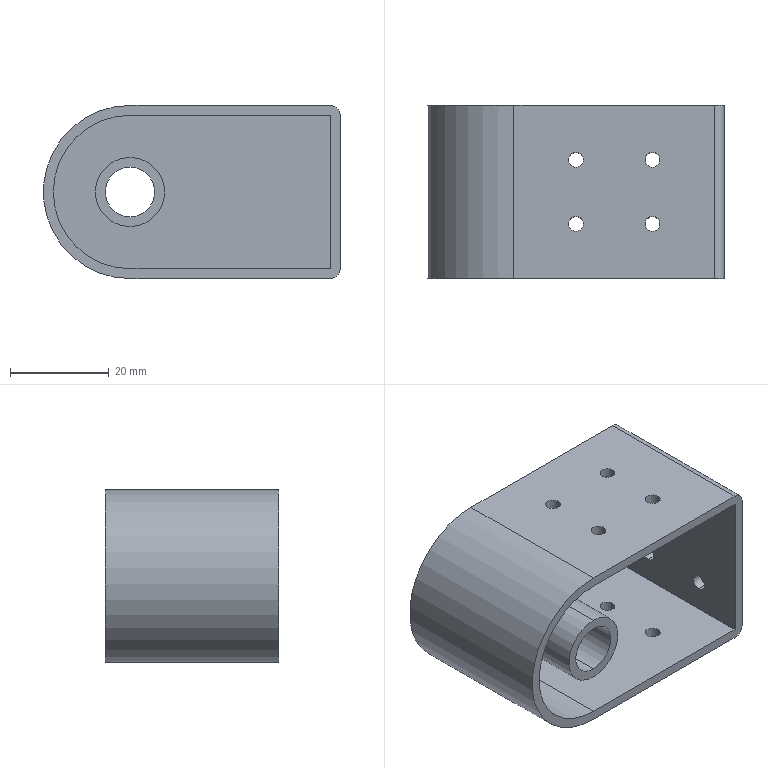Part | SolidWorks | features ICE 5, Extrusion 1, Fillet 1, Shell 1 | 1 solid | 42 faces | box 60 x 35 x 35 mm | volume 17116 mm3 | cylinder 32 | plane 10 | commonest cylinder face diameters 3 x24 4 x2 10 x2 14 x2 31 x1 35 x1
STEP:
#1=CARTESIAN_POINT('',(30.,24.748,-7.494));
#2=VERTEX_POINT('',#1);
#3=CARTESIAN_POINT('',(30.,24.748,-10.494));
#4=VERTEX_POINT('',#3);
#5=CARTESIAN_POINT('',(30.,24.748,-8.994));
#6=DIRECTION('',(1.,0.,0.));
#7=DIRECTION('',(0.,0.,1.));
#8=AXIS2_PLACEMENT_3D('',#5,#6,#7);
#9=CIRCLE('',#8,1.5);
#10=EDGE_CURVE('',#2,#4,#9,.T.);
#11=ORIENTED_EDGE('',*,*,#10,.T.);
#12=CARTESIAN_POINT('',(28.,24.748,-10.494));
#13=VERTEX_POINT('',#12);
#14=CARTESIAN_POINT('',(30.,24.748,-10.494));
#15=DIRECTION('',(-1.,0.,0.));
#16=VECTOR('',#15,1000.);
#17=LINE('',#14,#16);
#18=EDGE_CURVE('',#4,#13,#17,.T.);
#19=ORIENTED_EDGE('',*,*,#18,.T.);
#20=CARTESIAN_POINT('',(28.,24.748,-7.494));
#21=VERTEX_POINT('',#20);
#22=CARTESIAN_POINT('',(28.,24.748,-8.994));
#23=DIRECTION('',(1.,0.,0.));
#24=DIRECTION('',(0.,0.,1.));
#25=AXIS2_PLACEMENT_3D('',#22,#23,#24);
#26=CIRCLE('',#25,1.5);
#27=EDGE_CURVE('',#21,#13,#26,.T.);
#28=ORIENTED_EDGE('',*,*,#27,.F.);
#29=CARTESIAN_POINT('',(30.,24.748,-7.494));
#30=DIRECTION('',(-1.,0.,0.));
#31=VECTOR('',#30,1000.);
#32=LINE('',#29,#31);
#33=EDGE_CURVE('',#2,#21,#32,.T.);
#34=ORIENTED_EDGE('',*,*,#33,.F.);
#35=EDGE_LOOP('',(#11,#19,#28,#34));
#36=FACE_OUTER_BOUND('',#35,.T.);
#37=CARTESIAN_POINT('',(30.,24.748,-8.994));
#38=DIRECTION('',(-1.,0.,0.));
#39=DIRECTION('',(0.,0.,1.));
#40=AXIS2_PLACEMENT_3D('',#37,#38,#39);
#41=CYLINDRICAL_SURFACE('',#40,1.5);
#42=ADVANCED_FACE('',(#36),#41,.F.);
#43=CARTESIAN_POINT('',(30.,10.252,10.494));
#44=VERTEX_POINT('',#43);
#45=CARTESIAN_POINT('',(30.,10.252,7.494));
#46=VERTEX_POINT('',#45);
#47=CARTESIAN_POINT('',(30.,10.252,8.994));
#48=DIRECTION('',(1.,0.,0.));
#49=DIRECTION('',(0.,0.,1.));
#50=AXIS2_PLACEMENT_3D('',#47,#48,#49);
#51=CIRCLE('',#50,1.5);
#52=EDGE_CURVE('',#44,#46,#51,.T.);
#53=ORIENTED_EDGE('',*,*,#52,.T.);
#54=CARTESIAN_POINT('',(28.,10.252,7.494));
#55=VERTEX_POINT('',#54);
#56=CARTESIAN_POINT('',(30.,10.252,7.494));
#57=DIRECTION('',(-1.,0.,0.));
#58=VECTOR('',#57,1000.);
#59=LINE('',#56,#58);
#60=EDGE_CURVE('',#46,#55,#59,.T.);
#61=ORIENTED_EDGE('',*,*,#60,.T.);
#62=CARTESIAN_POINT('',(28.,10.252,10.494));
#63=VERTEX_POINT('',#62);
#64=CARTESIAN_POINT('',(28.,10.252,8.994));
#65=DIRECTION('',(1.,0.,0.));
#66=DIRECTION('',(0.,0.,1.));
#67=AXIS2_PLACEMENT_3D('',#64,#65,#66);
#68=CIRCLE('',#67,1.5);
#69=EDGE_CURVE('',#63,#55,#68,.T.);
#70=ORIENTED_EDGE('',*,*,#69,.F.);
#71=CARTESIAN_POINT('',(30.,10.252,10.494));
#72=DIRECTION('',(-1.,0.,0.));
#73=VECTOR('',#72,1000.);
#74=LINE('',#71,#73);
#75=EDGE_CURVE('',#44,#63,#74,.T.);
#76=ORIENTED_EDGE('',*,*,#75,.F.);
#77=EDGE_LOOP('',(#53,#61,#70,#76));
#78=FACE_OUTER_BOUND('',#77,.T.);
#79=CARTESIAN_POINT('',(30.,10.252,8.994));
#80=DIRECTION('',(-1.,0.,0.));
#81=DIRECTION('',(0.,0.,1.));
#82=AXIS2_PLACEMENT_3D('',#79,#80,#81);
#83=CYLINDRICAL_SURFACE('',#82,1.5);
#84=ADVANCED_FACE('',(#78),#83,.F.);
#85=CARTESIAN_POINT('',(30.,10.252,-7.494));
#86=VERTEX_POINT('',#85);
#87=CARTESIAN_POINT('',(30.,10.252,-10.494));
#88=VERTEX_POINT('',#87);
#89=CARTESIAN_POINT('',(30.,10.252,-8.994));
#90=DIRECTION('',(1.,0.,0.));
#91=DIRECTION('',(0.,0.,1.));
#92=AXIS2_PLACEMENT_3D('',#89,#90,#91);
#93=CIRCLE('',#92,1.5);
#94=EDGE_CURVE('',#86,#88,#93,.T.);
#95=ORIENTED_EDGE('',*,*,#94,.T.);
#96=CARTESIAN_POINT('',(28.,10.252,-10.494));
#97=VERTEX_POINT('',#96);
#98=CARTESIAN_POINT('',(30.,10.252,-10.494));
#99=DIRECTION('',(-1.,0.,0.));
#100=VECTOR('',#99,1000.);
#101=LINE('',#98,#100);
#102=EDGE_CURVE('',#88,#97,#101,.T.);
#103=ORIENTED_EDGE('',*,*,#102,.T.);
#104=CARTESIAN_POINT('',(28.,10.252,-7.494));
#105=VERTEX_POINT('',#104);
#106=CARTESIAN_POINT('',(28.,10.252,-8.994));
#107=DIRECTION('',(1.,0.,0.));
#108=DIRECTION('',(0.,0.,1.));
#109=AXIS2_PLACEMENT_3D('',#106,#107,#108);
#110=CIRCLE('',#109,1.5);
#111=EDGE_CURVE('',#105,#97,#110,.T.);
#112=ORIENTED_EDGE('',*,*,#111,.F.);
#113=CARTESIAN_POINT('',(30.,10.252,-7.494));
#114=DIRECTION('',(-1.,0.,0.));
#115=VECTOR('',#114,1000.);
#116=LINE('',#113,#115);
#117=EDGE_CURVE('',#86,#105,#116,.T.);
#118=ORIENTED_EDGE('',*,*,#117,.F.);
#119=EDGE_LOOP('',(#95,#103,#112,#118));
#120=FACE_OUTER_BOUND('',#119,.T.);
#121=CARTESIAN_POINT('',(30.,10.252,-8.994));
#122=DIRECTION('',(-1.,0.,0.));
#123=DIRECTION('',(0.,0.,1.));
#124=AXIS2_PLACEMENT_3D('',#121,#122,#123);
#125=CYLINDRICAL_SURFACE('',#124,1.5);
#126=ADVANCED_FACE('',(#120),#125,.F.);
#127=CARTESIAN_POINT('',(30.,24.748,10.494));
#128=VERTEX_POINT('',#127);
#129=CARTESIAN_POINT('',(30.,24.748,7.494));
#130=VERTEX_POINT('',#129);
#131=CARTESIAN_POINT('',(30.,24.748,8.994));
#132=DIRECTION('',(1.,0.,0.));
#133=DIRECTION('',(0.,0.,1.));
#134=AXIS2_PLACEMENT_3D('',#131,#132,#133);
#135=CIRCLE('',#134,1.5);
#136=EDGE_CURVE('',#128,#130,#135,.T.);
#137=ORIENTED_EDGE('',*,*,#136,.T.);
#138=CARTESIAN_POINT('',(28.,24.748,7.494));
#139=VERTEX_POINT('',#138);
#140=CARTESIAN_POINT('',(30.,24.748,7.494));
#141=DIRECTION('',(-1.,0.,0.));
#142=VECTOR('',#141,1000.);
#143=LINE('',#140,#142);
#144=EDGE_CURVE('',#130,#139,#143,.T.);
#145=ORIENTED_EDGE('',*,*,#144,.T.);
#146=CARTESIAN_POINT('',(28.,24.748,10.494));
#147=VERTEX_POINT('',#146);
#148=CARTESIAN_POINT('',(28.,24.748,8.994));
#149=DIRECTION('',(1.,0.,0.));
#150=DIRECTION('',(0.,0.,1.));
#151=AXIS2_PLACEMENT_3D('',#148,#149,#150);
#152=CIRCLE('',#151,1.5);
#153=EDGE_CURVE('',#147,#139,#152,.T.);
#154=ORIENTED_EDGE('',*,*,#153,.F.);
#155=CARTESIAN_POINT('',(30.,24.748,10.494));
#156=DIRECTION('',(-1.,0.,0.));
#157=VECTOR('',#156,1000.);
#158=LINE('',#155,#157);
#159=EDGE_CURVE('',#128,#147,#158,.T.);
#160=ORIENTED_EDGE('',*,*,#159,.F.);
#161=EDGE_LOOP('',(#137,#145,#154,#160));
#162=FACE_OUTER_BOUND('',#161,.T.);
#163=CARTESIAN_POINT('',(30.,24.748,8.994));
#164=DIRECTION('',(-1.,0.,0.));
#165=DIRECTION('',(0.,0.,1.));
#166=AXIS2_PLACEMENT_3D('',#163,#164,#165);
#167=CYLINDRICAL_SURFACE('',#166,1.5);
#168=ADVANCED_FACE('',(#162),#167,.F.);
#169=CARTESIAN_POINT('',(-1.5,11.017,-17.5));
#170=VERTEX_POINT('',#169);
#171=CARTESIAN_POINT('',(1.5,11.017,-17.5));
#172=VERTEX_POINT('',#171);
#173=CARTESIAN_POINT('',(0.,11.017,-17.5));
#174=DIRECTION('',(0.,0.,1.));
#175=DIRECTION('',(-1.,0.,0.));
#176=AXIS2_PLACEMENT_3D('',#173,#174,#175);
#177=CIRCLE('',#176,1.5);
#178=EDGE_CURVE('',#170,#172,#177,.T.);
#179=ORIENTED_EDGE('',*,*,#178,.F.);
#180=CARTESIAN_POINT('',(-1.5,11.017,-15.5));
#181=VERTEX_POINT('',#180);
#182=CARTESIAN_POINT('',(-1.5,11.017,-17.5));
#183=DIRECTION('',(0.,0.,1.));
#184=VECTOR('',#183,1000.);
#185=LINE('',#182,#184);
#186=EDGE_CURVE('',#170,#181,#185,.T.);
#187=ORIENTED_EDGE('',*,*,#186,.T.);
#188=CARTESIAN_POINT('',(1.5,11.017,-15.5));
#189=VERTEX_POINT('',#188);
#190=CARTESIAN_POINT('',(0.,11.017,-15.5));
#191=DIRECTION('',(0.,0.,1.));
#192=DIRECTION('',(1.,0.,0.));
#193=AXIS2_PLACEMENT_3D('',#190,#191,#192);
#194=CIRCLE('',#193,1.5);
#195=EDGE_CURVE('',#181,#189,#194,.T.);
#196=ORIENTED_EDGE('',*,*,#195,.T.);
#197=CARTESIAN_POINT('',(1.5,11.017,-17.5));
#198=DIRECTION('',(0.,0.,1.));
#199=VECTOR('',#198,1000.);
#200=LINE('',#197,#199);
#201=EDGE_CURVE('',#172,#189,#200,.T.);
#202=ORIENTED_EDGE('',*,*,#201,.F.);
#203=EDGE_LOOP('',(#179,#187,#196,#202));
#204=FACE_OUTER_BOUND('',#203,.T.);
#205=CARTESIAN_POINT('',(0.,11.017,-17.5));
#206=DIRECTION('',(0.,0.,1.));
#207=DIRECTION('',(1.,0.,0.));
#208=AXIS2_PLACEMENT_3D('',#205,#206,#207);
#209=CYLINDRICAL_SURFACE('',#208,1.5);
#210=ADVANCED_FACE('',(#204),#209,.F.);
#211=CARTESIAN_POINT('',(14.,11.017,-17.5));
#212=VERTEX_POINT('',#211);
#213=CARTESIAN_POINT('',(17.,11.017,-17.5));
#214=VERTEX_POINT('',#213);
#215=CARTESIAN_POINT('',(15.5,11.017,-17.5));
#216=DIRECTION('',(0.,0.,1.));
#217=DIRECTION('',(1.,0.,0.));
#218=AXIS2_PLACEMENT_3D('',#215,#216,#217);
#219=CIRCLE('',#218,1.5);
#220=EDGE_CURVE('',#212,#214,#219,.T.);
#221=ORIENTED_EDGE('',*,*,#220,.F.);
#222=CARTESIAN_POINT('',(14.,11.017,-15.5));
#223=VERTEX_POINT('',#222);
#224=CARTESIAN_POINT('',(14.,11.017,-17.5));
#225=DIRECTION('',(0.,0.,1.));
#226=VECTOR('',#225,1000.);
#227=LINE('',#224,#226);
#228=EDGE_CURVE('',#212,#223,#227,.T.);
#229=ORIENTED_EDGE('',*,*,#228,.T.);
#230=CARTESIAN_POINT('',(17.,11.017,-15.5));
#231=VERTEX_POINT('',#230);
#232=CARTESIAN_POINT('',(15.5,11.017,-15.5));
#233=DIRECTION('',(0.,0.,1.));
#234=DIRECTION('',(1.,0.,0.));
#235=AXIS2_PLACEMENT_3D('',#232,#233,#234);
#236=CIRCLE('',#235,1.5);
#237=EDGE_CURVE('',#223,#231,#236,.T.);
#238=ORIENTED_EDGE('',*,*,#237,.T.);
#239=CARTESIAN_POINT('',(17.,11.017,-17.5));
#240=DIRECTION('',(0.,0.,1.));
#241=VECTOR('',#240,1000.);
#242=LINE('',#239,#241);
#243=EDGE_CURVE('',#214,#231,#242,.T.);
#244=ORIENTED_EDGE('',*,*,#243,.F.);
#245=EDGE_LOOP('',(#221,#229,#238,#244));
#246=FACE_OUTER_BOUND('',#245,.T.);
#247=CARTESIAN_POINT('',(15.5,11.017,-17.5));
#248=DIRECTION('',(0.,0.,1.));
#249=DIRECTION('',(1.,0.,0.));
#250=AXIS2_PLACEMENT_3D('',#247,#248,#249);
#251=CYLINDRICAL_SURFACE('',#250,1.5);
#252=ADVANCED_FACE('',(#246),#251,.F.);
#253=CARTESIAN_POINT('',(14.,23.983,-17.5));
#254=VERTEX_POINT('',#253);
#255=CARTESIAN_POINT('',(17.,23.983,-17.5));
#256=VERTEX_POINT('',#255);
#257=CARTESIAN_POINT('',(15.5,23.983,-17.5));
#258=DIRECTION('',(0.,0.,1.));
#259=DIRECTION('',(-1.,0.,0.));
#260=AXIS2_PLACEMENT_3D('',#257,#258,#259);
#261=CIRCLE('',#260,1.5);
#262=EDGE_CURVE('',#254,#256,#261,.T.);
#263=ORIENTED_EDGE('',*,*,#262,.F.);
#264=CARTESIAN_POINT('',(14.,23.983,-15.5));
#265=VERTEX_POINT('',#264);
#266=CARTESIAN_POINT('',(14.,23.983,-17.5));
#267=DIRECTION('',(0.,0.,1.));
#268=VECTOR('',#267,1000.);
#269=LINE('',#266,#268);
#270=EDGE_CURVE('',#254,#265,#269,.T.);
#271=ORIENTED_EDGE('',*,*,#270,.T.);
#272=CARTESIAN_POINT('',(17.,23.983,-15.5));
#273=VERTEX_POINT('',#272);
#274=CARTESIAN_POINT('',(15.5,23.983,-15.5));
#275=DIRECTION('',(0.,0.,1.));
#276=DIRECTION('',(1.,0.,0.));
#277=AXIS2_PLACEMENT_3D('',#274,#275,#276);
#278=CIRCLE('',#277,1.5);
#279=EDGE_CURVE('',#265,#273,#278,.T.);
#280=ORIENTED_EDGE('',*,*,#279,.T.);
#281=CARTESIAN_POINT('',(17.,23.983,-17.5));
#282=DIRECTION('',(0.,0.,1.));
#283=VECTOR('',#282,1000.);
#284=LINE('',#281,#283);
#285=EDGE_CURVE('',#256,#273,#284,.T.);
#286=ORIENTED_EDGE('',*,*,#285,.F.);
#287=EDGE_LOOP('',(#263,#271,#280,#286));
#288=FACE_OUTER_BOUND('',#287,.T.);
#289=CARTESIAN_POINT('',(15.5,23.983,-17.5));
#290=DIRECTION('',(0.,0.,1.));
#291=DIRECTION('',(1.,0.,0.));
#292=AXIS2_PLACEMENT_3D('',#289,#290,#291);
#293=CYLINDRICAL_SURFACE('',#292,1.5);
#294=ADVANCED_FACE('',(#288),#293,.F.);
#295=CARTESIAN_POINT('',(-1.5,23.983,-17.5));
#296=VERTEX_POINT('',#295);
#297=CARTESIAN_POINT('',(1.5,23.983,-17.5));
#298=VERTEX_POINT('',#297);
#299=CARTESIAN_POINT('',(0.,23.983,-17.5));
#300=DIRECTION('',(0.,0.,1.));
#301=DIRECTION('',(1.,0.,0.));
#302=AXIS2_PLACEMENT_3D('',#299,#300,#301);
#303=CIRCLE('',#302,1.5);
#304=EDGE_CURVE('',#296,#298,#303,.T.);
#305=ORIENTED_EDGE('',*,*,#304,.F.);
#306=CARTESIAN_POINT('',(-1.5,23.983,-15.5));
#307=VERTEX_POINT('',#306);
#308=CARTESIAN_POINT('',(-1.5,23.983,-17.5));
#309=DIRECTION('',(0.,0.,1.));
#310=VECTOR('',#309,1000.);
#311=LINE('',#308,#310);
#312=EDGE_CURVE('',#296,#307,#311,.T.);
#313=ORIENTED_EDGE('',*,*,#312,.T.);
#314=CARTESIAN_POINT('',(1.5,23.983,-15.5));
#315=VERTEX_POINT('',#314);
#316=CARTESIAN_POINT('',(0.,23.983,-15.5));
#317=DIRECTION('',(0.,0.,1.));
#318=DIRECTION('',(1.,0.,0.));
#319=AXIS2_PLACEMENT_3D('',#316,#317,#318);
#320=CIRCLE('',#319,1.5);
#321=EDGE_CURVE('',#307,#315,#320,.T.);
#322=ORIENTED_EDGE('',*,*,#321,.T.);
#323=CARTESIAN_POINT('',(1.5,23.983,-17.5));
#324=DIRECTION('',(0.,0.,1.));
#325=VECTOR('',#324,1000.);
#326=LINE('',#323,#325);
#327=EDGE_CURVE('',#298,#315,#326,.T.);
#328=ORIENTED_EDGE('',*,*,#327,.F.);
#329=EDGE_LOOP('',(#305,#313,#322,#328));
#330=FACE_OUTER_BOUND('',#329,.T.);
#331=CARTESIAN_POINT('',(0.,23.983,-17.5));
#332=DIRECTION('',(0.,0.,1.));
#333=DIRECTION('',(1.,0.,0.));
#334=AXIS2_PLACEMENT_3D('',#331,#332,#333);
#335=CYLINDRICAL_SURFACE('',#334,1.5);
#336=ADVANCED_FACE('',(#330),#335,.F.);
#337=CARTESIAN_POINT('',(1.5,11.017,15.5));
#338=VERTEX_POINT('',#337);
#339=CARTESIAN_POINT('',(-1.5,11.017,15.5));
#340=VERTEX_POINT('',#339);
#341=CARTESIAN_POINT('',(0.,11.017,15.5));
#342=DIRECTION('',(0.,0.,-1.));
#343=DIRECTION('',(-1.,0.,0.));
#344=AXIS2_PLACEMENT_3D('',#341,#342,#343);
#345=CIRCLE('',#344,1.5);
#346=EDGE_CURVE('',#338,#340,#345,.T.);
#347=ORIENTED_EDGE('',*,*,#346,.T.);
#348=CARTESIAN_POINT('',(-1.5,11.017,17.5));
#349=VERTEX_POINT('',#348);
#350=CARTESIAN_POINT('',(-1.5,11.017,-17.5));
#351=DIRECTION('',(0.,0.,1.));
#352=VECTOR('',#351,1000.);
#353=LINE('',#350,#352);
#354=EDGE_CURVE('',#340,#349,#353,.T.);
#355=ORIENTED_EDGE('',*,*,#354,.T.);
#356=CARTESIAN_POINT('',(1.5,11.017,17.5));
#357=VERTEX_POINT('',#356);
#358=CARTESIAN_POINT('',(0.,11.017,17.5));
#359=DIRECTION('',(0.,0.,-1.));
#360=DIRECTION('',(-1.,0.,0.));
#361=AXIS2_PLACEMENT_3D('',#358,#359,#360);
#362=CIRCLE('',#361,1.5);
#363=EDGE_CURVE('',#357,#349,#362,.T.);
#364=ORIENTED_EDGE('',*,*,#363,.F.);
#365=CARTESIAN_POINT('',(1.5,11.017,-17.5));
#366=DIRECTION('',(0.,0.,1.));
#367=VECTOR('',#366,1000.);
#368=LINE('',#365,#367);
#369=EDGE_CURVE('',#338,#357,#368,.T.);
#370=ORIENTED_EDGE('',*,*,#369,.F.);
#371=EDGE_LOOP('',(#347,#355,#364,#370));
#372=FACE_OUTER_BOUND('',#371,.T.);
#373=CARTESIAN_POINT('',(0.,11.017,-17.5));
#374=DIRECTION('',(0.,0.,1.));
#375=DIRECTION('',(1.,0.,0.));
#376=AXIS2_PLACEMENT_3D('',#373,#374,#375);
#377=CYLINDRICAL_SURFACE('',#376,1.5);
#378=ADVANCED_FACE('',(#372),#377,.F.);
#379=CARTESIAN_POINT('',(17.,11.017,15.5));
#380=VERTEX_POINT('',#379);
#381=CARTESIAN_POINT('',(14.,11.017,15.5));
#382=VERTEX_POINT('',#381);
#383=CARTESIAN_POINT('',(15.5,11.017,15.5));
#384=DIRECTION('',(0.,0.,-1.));
#385=DIRECTION('',(-1.,0.,0.));
#386=AXIS2_PLACEMENT_3D('',#383,#384,#385);
#387=CIRCLE('',#386,1.5);
#388=EDGE_CURVE('',#380,#382,#387,.T.);
#389=ORIENTED_EDGE('',*,*,#388,.T.);
#390=CARTESIAN_POINT('',(14.,11.017,17.5));
#391=VERTEX_POINT('',#390);
#392=CARTESIAN_POINT('',(14.,11.017,-17.5));
#393=DIRECTION('',(0.,0.,1.));
#394=VECTOR('',#393,1000.);
#395=LINE('',#392,#394);
#396=EDGE_CURVE('',#382,#391,#395,.T.);
#397=ORIENTED_EDGE('',*,*,#396,.T.);
#398=CARTESIAN_POINT('',(17.,11.017,17.5));
#399=VERTEX_POINT('',#398);
#400=CARTESIAN_POINT('',(15.5,11.017,17.5));
#401=DIRECTION('',(0.,0.,-1.));
#402=DIRECTION('',(-1.,0.,0.));
#403=AXIS2_PLACEMENT_3D('',#400,#401,#402);
#404=CIRCLE('',#403,1.5);
#405=EDGE_CURVE('',#399,#391,#404,.T.);
#406=ORIENTED_EDGE('',*,*,#405,.F.);
#407=CARTESIAN_POINT('',(17.,11.017,-17.5));
#408=DIRECTION('',(0.,0.,1.));
#409=VECTOR('',#408,1000.);
#410=LINE('',#407,#409);
#411=EDGE_CURVE('',#380,#399,#410,.T.);
#412=ORIENTED_EDGE('',*,*,#411,.F.);
#413=EDGE_LOOP('',(#389,#397,#406,#412));
#414=FACE_OUTER_BOUND('',#413,.T.);
#415=CARTESIAN_POINT('',(15.5,11.017,-17.5));
#416=DIRECTION('',(0.,0.,1.));
#417=DIRECTION('',(1.,0.,0.));
#418=AXIS2_PLACEMENT_3D('',#415,#416,#417);
#419=CYLINDRICAL_SURFACE('',#418,1.5);
#420=ADVANCED_FACE('',(#414),#419,.F.);
#421=CARTESIAN_POINT('',(17.,23.983,15.5));
#422=VERTEX_POINT('',#421);
#423=CARTESIAN_POINT('',(14.,23.983,15.5));
#424=VERTEX_POINT('',#423);
#425=CARTESIAN_POINT('',(15.5,23.983,15.5));
#426=DIRECTION('',(0.,0.,-1.));
#427=DIRECTION('',(-1.,0.,0.));
#428=AXIS2_PLACEMENT_3D('',#425,#426,#427);
#429=CIRCLE('',#428,1.5);
#430=EDGE_CURVE('',#422,#424,#429,.T.);
#431=ORIENTED_EDGE('',*,*,#430,.T.);
#432=CARTESIAN_POINT('',(14.,23.983,17.5));
#433=VERTEX_POINT('',#432);
#434=CARTESIAN_POINT('',(14.,23.983,-17.5));
#435=DIRECTION('',(0.,0.,1.));
#436=VECTOR('',#435,1000.);
#437=LINE('',#434,#436);
#438=EDGE_CURVE('',#424,#433,#437,.T.);
#439=ORIENTED_EDGE('',*,*,#438,.T.);
#440=CARTESIAN_POINT('',(17.,23.983,17.5));
#441=VERTEX_POINT('',#440);
#442=CARTESIAN_POINT('',(15.5,23.983,17.5));
#443=DIRECTION('',(0.,0.,-1.));
#444=DIRECTION('',(-1.,0.,0.));
#445=AXIS2_PLACEMENT_3D('',#442,#443,#444);
#446=CIRCLE('',#445,1.5);
#447=EDGE_CURVE('',#441,#433,#446,.T.);
#448=ORIENTED_EDGE('',*,*,#447,.F.);
#449=CARTESIAN_POINT('',(17.,23.983,-17.5));
#450=DIRECTION('',(0.,0.,1.));
#451=VECTOR('',#450,1000.);
#452=LINE('',#449,#451);
#453=EDGE_CURVE('',#422,#441,#452,.T.);
#454=ORIENTED_EDGE('',*,*,#453,.F.);
#455=EDGE_LOOP('',(#431,#439,#448,#454));
#456=FACE_OUTER_BOUND('',#455,.T.);
#457=CARTESIAN_POINT('',(15.5,23.983,-17.5));
#458=DIRECTION('',(0.,0.,1.));
#459=DIRECTION('',(1.,0.,0.));
#460=AXIS2_PLACEMENT_3D('',#457,#458,#459);
#461=CYLINDRICAL_SURFACE('',#460,1.5);
#462=ADVANCED_FACE('',(#456),#461,.F.);
#463=CARTESIAN_POINT('',(1.5,23.983,15.5));
#464=VERTEX_POINT('',#463);
#465=CARTESIAN_POINT('',(-1.5,23.983,15.5));
#466=VERTEX_POINT('',#465);
#467=CARTESIAN_POINT('',(0.,23.983,15.5));
#468=DIRECTION('',(0.,0.,-1.));
#469=DIRECTION('',(-1.,0.,0.));
#470=AXIS2_PLACEMENT_3D('',#467,#468,#469);
#471=CIRCLE('',#470,1.5);
#472=EDGE_CURVE('',#464,#466,#471,.T.);
#473=ORIENTED_EDGE('',*,*,#472,.T.);
#474=CARTESIAN_POINT('',(-1.5,23.983,17.5));
#475=VERTEX_POINT('',#474);
#476=CARTESIAN_POINT('',(-1.5,23.983,-17.5));
#477=DIRECTION('',(0.,0.,1.));
#478=VECTOR('',#477,1000.);
#479=LINE('',#476,#478);
#480=EDGE_CURVE('',#466,#475,#479,.T.);
#481=ORIENTED_EDGE('',*,*,#480,.T.);
#482=CARTESIAN_POINT('',(1.5,23.983,17.5));
#483=VERTEX_POINT('',#482);
#484=CARTESIAN_POINT('',(0.,23.983,17.5));
#485=DIRECTION('',(0.,0.,-1.));
#486=DIRECTION('',(-1.,0.,0.));
#487=AXIS2_PLACEMENT_3D('',#484,#485,#486);
#488=CIRCLE('',#487,1.5);
#489=EDGE_CURVE('',#483,#475,#488,.T.);
#490=ORIENTED_EDGE('',*,*,#489,.F.);
#491=CARTESIAN_POINT('',(1.5,23.983,-17.5));
#492=DIRECTION('',(0.,0.,1.));
#493=VECTOR('',#492,1000.);
#494=LINE('',#491,#493);
#495=EDGE_CURVE('',#464,#483,#494,.T.);
#496=ORIENTED_EDGE('',*,*,#495,.F.);
#497=EDGE_LOOP('',(#473,#481,#490,#496));
#498=FACE_OUTER_BOUND('',#497,.T.);
#499=CARTESIAN_POINT('',(0.,23.983,-17.5));
#500=DIRECTION('',(0.,0.,1.));
#501=DIRECTION('',(1.,0.,0.));
#502=AXIS2_PLACEMENT_3D('',#499,#500,#501);
#503=CYLINDRICAL_SURFACE('',#502,1.5);
#504=ADVANCED_FACE('',(#498),#503,.F.);
#505=CARTESIAN_POINT('',(-12.5,0.,7.));
#506=VERTEX_POINT('',#505);
#507=CARTESIAN_POINT('',(-12.5,0.,-7.));
#508=VERTEX_POINT('',#507);
#509=CARTESIAN_POINT('',(-12.5,0.,0.));
#510=DIRECTION('',(0.,1.,0.));
#511=DIRECTION('',(0.,0.,-1.));
#512=AXIS2_PLACEMENT_3D('',#509,#510,#511);
#513=CIRCLE('',#512,7.);
#514=EDGE_CURVE('',#506,#508,#513,.T.);
#515=ORIENTED_EDGE('',*,*,#514,.T.);
#516=CARTESIAN_POINT('',(-12.5,33.,-7.));
#517=VERTEX_POINT('',#516);
#518=CARTESIAN_POINT('',(-12.5,0.,-7.));
#519=DIRECTION('',(0.,1.,0.));
#520=VECTOR('',#519,1000.);
#521=LINE('',#518,#520);
#522=EDGE_CURVE('',#508,#517,#521,.T.);
#523=ORIENTED_EDGE('',*,*,#522,.T.);
#524=CARTESIAN_POINT('',(-12.5,33.,7.));
#525=VERTEX_POINT('',#524);
#526=CARTESIAN_POINT('',(-12.5,33.,0.));
#527=DIRECTION('',(0.,1.,0.));
#528=DIRECTION('',(0.,0.,-1.));
#529=AXIS2_PLACEMENT_3D('',#526,#527,#528);
#530=CIRCLE('',#529,7.);
#531=EDGE_CURVE('',#525,#517,#530,.T.);
#532=ORIENTED_EDGE('',*,*,#531,.F.);
#533=CARTESIAN_POINT('',(-12.5,0.,7.));
#534=DIRECTION('',(0.,1.,0.));
#535=VECTOR('',#534,1000.);
#536=LINE('',#533,#535);
#537=EDGE_CURVE('',#506,#525,#536,.T.);
#538=ORIENTED_EDGE('',*,*,#537,.F.);
#539=EDGE_LOOP('',(#515,#523,#532,#538));
#540=FACE_OUTER_BOUND('',#539,.T.);
#541=CARTESIAN_POINT('',(-12.5,0.,0.));
#542=DIRECTION('',(0.,1.,0.));
#543=DIRECTION('',(0.,0.,1.));
#544=AXIS2_PLACEMENT_3D('',#541,#542,#543);
#545=CYLINDRICAL_SURFACE('',#544,7.);
#546=ADVANCED_FACE('',(#540),#545,.T.);
#547=CARTESIAN_POINT('',(-12.5,0.,-5.));
#548=VERTEX_POINT('',#547);
#549=CARTESIAN_POINT('',(-12.5,0.,5.));
#550=VERTEX_POINT('',#549);
#551=CARTESIAN_POINT('',(-12.5,0.,0.));
#552=DIRECTION('',(0.,1.,0.));
#553=DIRECTION('',(0.,0.,1.));
#554=AXIS2_PLACEMENT_3D('',#551,#552,#553);
#555=CIRCLE('',#554,5.);
#556=EDGE_CURVE('',#548,#550,#555,.T.);
#557=ORIENTED_EDGE('',*,*,#556,.F.);
#558=CARTESIAN_POINT('',(-12.5,35.,-5.));
#559=VERTEX_POINT('',#558);
#560=CARTESIAN_POINT('',(-12.5,0.,-5.));
#561=DIRECTION('',(0.,1.,0.));
#562=VECTOR('',#561,1000.);
#563=LINE('',#560,#562);
#564=EDGE_CURVE('',#548,#559,#563,.T.);
#565=ORIENTED_EDGE('',*,*,#564,.T.);
#566=CARTESIAN_POINT('',(-12.5,35.,5.));
#567=VERTEX_POINT('',#566);
#568=CARTESIAN_POINT('',(-12.5,35.,0.));
#569=DIRECTION('',(0.,1.,0.));
#570=DIRECTION('',(0.,0.,1.));
#571=AXIS2_PLACEMENT_3D('',#568,#569,#570);
#572=CIRCLE('',#571,5.);
#573=EDGE_CURVE('',#559,#567,#572,.T.);
#574=ORIENTED_EDGE('',*,*,#573,.T.);
#575=CARTESIAN_POINT('',(-12.5,0.,5.));
#576=DIRECTION('',(0.,1.,0.));
#577=VECTOR('',#576,1000.);
#578=LINE('',#575,#577);
#579=EDGE_CURVE('',#550,#567,#578,.T.);
#580=ORIENTED_EDGE('',*,*,#579,.F.);
#581=EDGE_LOOP('',(#557,#565,#574,#580));
#582=FACE_OUTER_BOUND('',#581,.T.);
#583=CARTESIAN_POINT('',(-12.5,0.,0.));
#584=DIRECTION('',(0.,1.,0.));
#585=DIRECTION('',(0.,0.,1.));
#586=AXIS2_PLACEMENT_3D('',#583,#584,#585);
#587=CYLINDRICAL_SURFACE('',#586,5.);
#588=ADVANCED_FACE('',(#582),#587,.F.);
#589=CARTESIAN_POINT('',(28.,0.,-17.5));
#590=VERTEX_POINT('',#589);
#591=CARTESIAN_POINT('',(-12.5,0.,-17.5));
#592=VERTEX_POINT('',#591);
#593=CARTESIAN_POINT('',(-30.,0.,-17.5));
#594=DIRECTION('',(-1.,0.,0.));
#595=VECTOR('',#594,1000.);
#596=LINE('',#593,#595);
#597=EDGE_CURVE('',#590,#592,#596,.T.);
#598=ORIENTED_EDGE('',*,*,#597,.F.);
#599=CARTESIAN_POINT('',(30.,0.,-15.5));
#600=VERTEX_POINT('',#599);
#601=CARTESIAN_POINT('',(28.,0.,-15.5));
#602=DIRECTION('',(0.,-1.,0.));
#603=DIRECTION('',(0.,0.,-1.));
#604=AXIS2_PLACEMENT_3D('',#601,#602,#603);
#605=CIRCLE('',#604,2.);
#606=EDGE_CURVE('',#590,#600,#605,.T.);
#607=ORIENTED_EDGE('',*,*,#606,.T.);
#608=CARTESIAN_POINT('',(30.,0.,15.5));
#609=VERTEX_POINT('',#608);
#610=CARTESIAN_POINT('',(30.,0.,17.5));
#611=DIRECTION('',(0.,0.,-1.));
#612=VECTOR('',#611,1000.);
#613=LINE('',#610,#612);
#614=EDGE_CURVE('',#609,#600,#613,.T.);
#615=ORIENTED_EDGE('',*,*,#614,.F.);
#616=CARTESIAN_POINT('',(28.,0.,17.5));
#617=VERTEX_POINT('',#616);
#618=CARTESIAN_POINT('',(28.,0.,15.5));
#619=DIRECTION('',(0.,-1.,0.));
#620=DIRECTION('',(0.,0.,-1.));
#621=AXIS2_PLACEMENT_3D('',#618,#619,#620);
#622=CIRCLE('',#621,2.);
#623=EDGE_CURVE('',#609,#617,#622,.T.);
#624=ORIENTED_EDGE('',*,*,#623,.T.);
#625=CARTESIAN_POINT('',(-12.5,0.,17.5));
#626=VERTEX_POINT('',#625);
#627=CARTESIAN_POINT('',(-30.,0.,17.5));
#628=DIRECTION('',(1.,0.,0.));
#629=VECTOR('',#628,1000.);
#630=LINE('',#627,#629);
#631=EDGE_CURVE('',#626,#617,#630,.T.);
#632=ORIENTED_EDGE('',*,*,#631,.F.);
#633=CARTESIAN_POINT('',(-12.5,0.,0.));
#634=DIRECTION('',(0.,-1.,0.));
#635=DIRECTION('',(0.,0.,1.));
#636=AXIS2_PLACEMENT_3D('',#633,#634,#635);
#637=CIRCLE('',#636,17.5);
#638=EDGE_CURVE('',#626,#592,#637,.T.);
#639=ORIENTED_EDGE('',*,*,#638,.T.);
#640=EDGE_LOOP('',(#598,#607,#615,#624,#632,#639));
#641=FACE_OUTER_BOUND('',#640,.T.);
#642=CARTESIAN_POINT('',(28.,0.,15.5));
#643=VERTEX_POINT('',#642);
#644=CARTESIAN_POINT('',(28.,0.,-15.5));
#645=VERTEX_POINT('',#644);
#646=CARTESIAN_POINT('',(28.,0.,0.));
#647=DIRECTION('',(0.,0.,-1.));
#648=VECTOR('',#647,1000.);
#649=LINE('',#646,#648);
#650=EDGE_CURVE('',#643,#645,#649,.T.);
#651=ORIENTED_EDGE('',*,*,#650,.T.);
#652=CARTESIAN_POINT('',(-12.5,0.,-15.5));
#653=VERTEX_POINT('',#652);
#654=CARTESIAN_POINT('',(0.,0.,-15.5));
#655=DIRECTION('',(-1.,0.,0.));
#656=VECTOR('',#655,1000.);
#657=LINE('',#654,#656);
#658=EDGE_CURVE('',#645,#653,#657,.T.);
#659=ORIENTED_EDGE('',*,*,#658,.T.);
#660=CARTESIAN_POINT('',(-12.5,0.,15.5));
#661=VERTEX_POINT('',#660);
#662=CARTESIAN_POINT('',(-12.5,0.,0.));
#663=DIRECTION('',(0.,-1.,0.));
#664=DIRECTION('',(0.,0.,-1.));
#665=AXIS2_PLACEMENT_3D('',#662,#663,#664);
#666=CIRCLE('',#665,15.5);
#667=EDGE_CURVE('',#661,#653,#666,.T.);
#668=ORIENTED_EDGE('',*,*,#667,.F.);
#669=CARTESIAN_POINT('',(0.,0.,15.5));
#670=DIRECTION('',(1.,0.,0.));
#671=VECTOR('',#670,1000.);
#672=LINE('',#669,#671);
#673=EDGE_CURVE('',#661,#643,#672,.T.);
#674=ORIENTED_EDGE('',*,*,#673,.T.);
#675=EDGE_LOOP('',(#651,#659,#668,#674));
#676=FACE_BOUND('',#675,.T.);
#677=CARTESIAN_POINT('',(0.,0.,0.));
#678=DIRECTION('',(0.,-1.,0.));
#679=DIRECTION('',(0.,0.,-1.));
#680=AXIS2_PLACEMENT_3D('',#677,#678,#679);
#681=PLANE('',#680);
#682=ADVANCED_FACE('',(#641,#676),#681,.T.);
#683=CARTESIAN_POINT('',(0.,11.017,-17.5));
#684=DIRECTION('',(0.,0.,1.));
#685=DIRECTION('',(-1.,0.,0.));
#686=AXIS2_PLACEMENT_3D('',#683,#684,#685);
#687=CIRCLE('',#686,1.5);
#688=EDGE_CURVE('',#172,#170,#687,.T.);
#689=ORIENTED_EDGE('',*,*,#688,.T.);
#690=ORIENTED_EDGE('',*,*,#178,.T.);
#691=EDGE_LOOP('',(#689,#690));
#692=FACE_BOUND('',#691,.T.);
#693=CARTESIAN_POINT('',(15.5,11.017,-17.5));
#694=DIRECTION('',(0.,0.,1.));
#695=DIRECTION('',(1.,0.,0.));
#696=AXIS2_PLACEMENT_3D('',#693,#694,#695);
#697=CIRCLE('',#696,1.5);
#698=EDGE_CURVE('',#214,#212,#697,.T.);
#699=ORIENTED_EDGE('',*,*,#698,.T.);
#700=ORIENTED_EDGE('',*,*,#220,.T.);
#701=EDGE_LOOP('',(#699,#700));
#702=FACE_BOUND('',#701,.T.);
#703=CARTESIAN_POINT('',(15.5,23.983,-17.5));
#704=DIRECTION('',(0.,0.,1.));
#705=DIRECTION('',(-1.,0.,0.));
#706=AXIS2_PLACEMENT_3D('',#703,#704,#705);
#707=CIRCLE('',#706,1.5);
#708=EDGE_CURVE('',#256,#254,#707,.T.);
#709=ORIENTED_EDGE('',*,*,#708,.T.);
#710=ORIENTED_EDGE('',*,*,#262,.T.);
#711=EDGE_LOOP('',(#709,#710));
#712=FACE_BOUND('',#711,.T.);
#713=CARTESIAN_POINT('',(0.,23.983,-17.5));
#714=DIRECTION('',(0.,0.,1.));
#715=DIRECTION('',(1.,0.,0.));
#716=AXIS2_PLACEMENT_3D('',#713,#714,#715);
#717=CIRCLE('',#716,1.5);
#718=EDGE_CURVE('',#298,#296,#717,.T.);
#719=ORIENTED_EDGE('',*,*,#718,.T.);
#720=ORIENTED_EDGE('',*,*,#304,.T.);
#721=EDGE_LOOP('',(#719,#720));
#722=FACE_BOUND('',#721,.T.);
#723=CARTESIAN_POINT('',(28.,35.,-17.5));
#724=VERTEX_POINT('',#723);
#725=CARTESIAN_POINT('',(-12.5,35.,-17.5));
#726=VERTEX_POINT('',#725);
#727=CARTESIAN_POINT('',(-30.,35.,-17.5));
#728=DIRECTION('',(-1.,0.,0.));
#729=VECTOR('',#728,1000.);
#730=LINE('',#727,#729);
#731=EDGE_CURVE('',#724,#726,#730,.T.);
#732=ORIENTED_EDGE('',*,*,#731,.F.);
#733=CARTESIAN_POINT('',(28.,35.,-17.5));
#734=DIRECTION('',(0.,-1.,0.));
#735=VECTOR('',#734,1000.);
#736=LINE('',#733,#735);
#737=EDGE_CURVE('',#724,#590,#736,.T.);
#738=ORIENTED_EDGE('',*,*,#737,.T.);
#739=ORIENTED_EDGE('',*,*,#597,.T.);
#740=CARTESIAN_POINT('',(-12.5,0.,-17.5));
#741=DIRECTION('',(0.,1.,0.));
#742=VECTOR('',#741,1000.);
#743=LINE('',#740,#742);
#744=EDGE_CURVE('',#592,#726,#743,.T.);
#745=ORIENTED_EDGE('',*,*,#744,.T.);
#746=EDGE_LOOP('',(#732,#738,#739,#745));
#747=FACE_OUTER_BOUND('',#746,.T.);
#748=CARTESIAN_POINT('',(-30.,35.,-17.5));
#749=DIRECTION('',(0.,0.,1.));
#750=DIRECTION('',(1.,0.,0.));
#751=AXIS2_PLACEMENT_3D('',#748,#749,#750);
#752=PLANE('',#751);
#753=ADVANCED_FACE('',(#692,#702,#712,#722,#747),#752,.F.);
#754=ORIENTED_EDGE('',*,*,#10,.F.);
#755=CARTESIAN_POINT('',(30.,24.748,-8.994));
#756=DIRECTION('',(1.,0.,0.));
#757=DIRECTION('',(0.,0.,1.));
#758=AXIS2_PLACEMENT_3D('',#755,#756,#757);
#759=CIRCLE('',#758,1.5);
#760=EDGE_CURVE('',#4,#2,#759,.T.);
#761=ORIENTED_EDGE('',*,*,#760,.F.);
#762=EDGE_LOOP('',(#754,#761));
#763=FACE_BOUND('',#762,.T.);
#764=ORIENTED_EDGE('',*,*,#52,.F.);
#765=CARTESIAN_POINT('',(30.,10.252,8.994));
#766=DIRECTION('',(1.,0.,0.));
#767=DIRECTION('',(0.,0.,1.));
#768=AXIS2_PLACEMENT_3D('',#765,#766,#767);
#769=CIRCLE('',#768,1.5);
#770=EDGE_CURVE('',#46,#44,#769,.T.);
#771=ORIENTED_EDGE('',*,*,#770,.F.);
#772=EDGE_LOOP('',(#764,#771));
#773=FACE_BOUND('',#772,.T.);
#774=ORIENTED_EDGE('',*,*,#94,.F.);
#775=CARTESIAN_POINT('',(30.,10.252,-8.994));
#776=DIRECTION('',(1.,0.,0.));
#777=DIRECTION('',(0.,0.,1.));
#778=AXIS2_PLACEMENT_3D('',#775,#776,#777);
#779=CIRCLE('',#778,1.5);
#780=EDGE_CURVE('',#88,#86,#779,.T.);
#781=ORIENTED_EDGE('',*,*,#780,.F.);
#782=EDGE_LOOP('',(#774,#781));
#783=FACE_BOUND('',#782,.T.);
#784=ORIENTED_EDGE('',*,*,#136,.F.);
#785=CARTESIAN_POINT('',(30.,24.748,8.994));
#786=DIRECTION('',(1.,0.,0.));
#787=DIRECTION('',(0.,0.,1.));
#788=AXIS2_PLACEMENT_3D('',#785,#786,#787);
#789=CIRCLE('',#788,1.5);
#790=EDGE_CURVE('',#130,#128,#789,.T.);
#791=ORIENTED_EDGE('',*,*,#790,.F.);
#792=EDGE_LOOP('',(#784,#791));
#793=FACE_BOUND('',#792,.T.);
#794=ORIENTED_EDGE('',*,*,#614,.T.);
#795=CARTESIAN_POINT('',(30.,35.,-15.5));
#796=VERTEX_POINT('',#795);
#797=CARTESIAN_POINT('',(30.,35.,-15.5));
#798=DIRECTION('',(0.,1.,0.));
#799=VECTOR('',#798,1000.);
#800=LINE('',#797,#799);
#801=EDGE_CURVE('',#600,#796,#800,.T.);
#802=ORIENTED_EDGE('',*,*,#801,.T.);
#803=CARTESIAN_POINT('',(30.,35.,15.5));
#804=VERTEX_POINT('',#803);
#805=CARTESIAN_POINT('',(30.,35.,17.5));
#806=DIRECTION('',(0.,0.,-1.));
#807=VECTOR('',#806,1000.);
#808=LINE('',#805,#807);
#809=EDGE_CURVE('',#804,#796,#808,.T.);
#810=ORIENTED_EDGE('',*,*,#809,.F.);
#811=CARTESIAN_POINT('',(30.,35.,15.5));
#812=DIRECTION('',(0.,-1.,0.));
#813=VECTOR('',#812,1000.);
#814=LINE('',#811,#813);
#815=EDGE_CURVE('',#804,#609,#814,.T.);
#816=ORIENTED_EDGE('',*,*,#815,.T.);
#817=EDGE_LOOP('',(#794,#802,#810,#816));
#818=FACE_OUTER_BOUND('',#817,.T.);
#819=CARTESIAN_POINT('',(30.,35.,17.5));
#820=DIRECTION('',(-1.,0.,0.));
#821=DIRECTION('',(0.,0.,1.));
#822=AXIS2_PLACEMENT_3D('',#819,#820,#821);
#823=PLANE('',#822);
#824=ADVANCED_FACE('',(#763,#773,#783,#793,#818),#823,.F.);
#825=ORIENTED_EDGE('',*,*,#363,.T.);
#826=CARTESIAN_POINT('',(0.,11.017,17.5));
#827=DIRECTION('',(0.,0.,-1.));
#828=DIRECTION('',(-1.,0.,0.));
#829=AXIS2_PLACEMENT_3D('',#826,#827,#828);
#830=CIRCLE('',#829,1.5);
#831=EDGE_CURVE('',#349,#357,#830,.T.);
#832=ORIENTED_EDGE('',*,*,#831,.T.);
#833=EDGE_LOOP('',(#825,#832));
#834=FACE_BOUND('',#833,.T.);
#835=ORIENTED_EDGE('',*,*,#405,.T.);
#836=CARTESIAN_POINT('',(15.5,11.017,17.5));
#837=DIRECTION('',(0.,0.,-1.));
#838=DIRECTION('',(-1.,0.,0.));
#839=AXIS2_PLACEMENT_3D('',#836,#837,#838);
#840=CIRCLE('',#839,1.5);
#841=EDGE_CURVE('',#391,#399,#840,.T.);
#842=ORIENTED_EDGE('',*,*,#841,.T.);
#843=EDGE_LOOP('',(#835,#842));
#844=FACE_BOUND('',#843,.T.);
#845=ORIENTED_EDGE('',*,*,#447,.T.);
#846=CARTESIAN_POINT('',(15.5,23.983,17.5));
#847=DIRECTION('',(0.,0.,-1.));
#848=DIRECTION('',(-1.,0.,0.));
#849=AXIS2_PLACEMENT_3D('',#846,#847,#848);
#850=CIRCLE('',#849,1.5);
#851=EDGE_CURVE('',#433,#441,#850,.T.);
#852=ORIENTED_EDGE('',*,*,#851,.T.);
#853=EDGE_LOOP('',(#845,#852));
#854=FACE_BOUND('',#853,.T.);
#855=ORIENTED_EDGE('',*,*,#489,.T.);
#856=CARTESIAN_POINT('',(0.,23.983,17.5));
#857=DIRECTION('',(0.,0.,-1.));
#858=DIRECTION('',(-1.,0.,0.));
#859=AXIS2_PLACEMENT_3D('',#856,#857,#858);
#860=CIRCLE('',#859,1.5);
#861=EDGE_CURVE('',#475,#483,#860,.T.);
#862=ORIENTED_EDGE('',*,*,#861,.T.);
#863=EDGE_LOOP('',(#855,#862));
#864=FACE_BOUND('',#863,.T.);
#865=ORIENTED_EDGE('',*,*,#631,.T.);
#866=CARTESIAN_POINT('',(28.,35.,17.5));
#867=VERTEX_POINT('',#866);
#868=CARTESIAN_POINT('',(28.,35.,17.5));
#869=DIRECTION('',(0.,1.,0.));
#870=VECTOR('',#869,1000.);
#871=LINE('',#868,#870);
#872=EDGE_CURVE('',#617,#867,#871,.T.);
#873=ORIENTED_EDGE('',*,*,#872,.T.);
#874=CARTESIAN_POINT('',(-12.5,35.,17.5));
#875=VERTEX_POINT('',#874);
#876=CARTESIAN_POINT('',(-30.,35.,17.5));
#877=DIRECTION('',(1.,0.,0.));
#878=VECTOR('',#877,1000.);
#879=LINE('',#876,#878);
#880=EDGE_CURVE('',#875,#867,#879,.T.);
#881=ORIENTED_EDGE('',*,*,#880,.F.);
#882=CARTESIAN_POINT('',(-12.5,0.,17.5));
#883=DIRECTION('',(0.,1.,0.));
#884=VECTOR('',#883,1000.);
#885=LINE('',#882,#884);
#886=EDGE_CURVE('',#626,#875,#885,.T.);
#887=ORIENTED_EDGE('',*,*,#886,.F.);
#888=EDGE_LOOP('',(#865,#873,#881,#887));
#889=FACE_OUTER_BOUND('',#888,.T.);
#890=CARTESIAN_POINT('',(-30.,35.,17.5));
#891=DIRECTION('',(0.,0.,-1.));
#892=DIRECTION('',(-1.,0.,0.));
#893=AXIS2_PLACEMENT_3D('',#890,#891,#892);
#894=PLANE('',#893);
#895=ADVANCED_FACE('',(#834,#844,#854,#864,#889),#894,.F.);
#896=CARTESIAN_POINT('',(-12.5,35.,0.));
#897=DIRECTION('',(0.,1.,0.));
#898=DIRECTION('',(0.,0.,1.));
#899=AXIS2_PLACEMENT_3D('',#896,#897,#898);
#900=CIRCLE('',#899,5.);
#901=EDGE_CURVE('',#567,#559,#900,.T.);
#902=ORIENTED_EDGE('',*,*,#901,.F.);
#903=ORIENTED_EDGE('',*,*,#573,.F.);
#904=EDGE_LOOP('',(#902,#903));
#905=FACE_BOUND('',#904,.T.);
#906=ORIENTED_EDGE('',*,*,#809,.T.);
#907=CARTESIAN_POINT('',(28.,35.,-15.5));
#908=DIRECTION('',(0.,1.,0.));
#909=DIRECTION('',(0.,0.,-1.));
#910=AXIS2_PLACEMENT_3D('',#907,#908,#909);
#911=CIRCLE('',#910,2.);
#912=EDGE_CURVE('',#796,#724,#911,.T.);
#913=ORIENTED_EDGE('',*,*,#912,.T.);
#914=ORIENTED_EDGE('',*,*,#731,.T.);
#915=CARTESIAN_POINT('',(-12.5,35.,0.));
#916=DIRECTION('',(0.,-1.,0.));
#917=DIRECTION('',(0.,0.,1.));
#918=AXIS2_PLACEMENT_3D('',#915,#916,#917);
#919=CIRCLE('',#918,17.5);
#920=EDGE_CURVE('',#875,#726,#919,.T.);
#921=ORIENTED_EDGE('',*,*,#920,.F.);
#922=ORIENTED_EDGE('',*,*,#880,.T.);
#923=CARTESIAN_POINT('',(28.,35.,15.5));
#924=DIRECTION('',(0.,1.,0.));
#925=DIRECTION('',(0.,0.,-1.));
#926=AXIS2_PLACEMENT_3D('',#923,#924,#925);
#927=CIRCLE('',#926,2.);
#928=EDGE_CURVE('',#867,#804,#927,.T.);
#929=ORIENTED_EDGE('',*,*,#928,.T.);
#930=EDGE_LOOP('',(#906,#913,#914,#921,#922,#929));
#931=FACE_OUTER_BOUND('',#930,.T.);
#932=CARTESIAN_POINT('',(0.,35.,0.));
#933=DIRECTION('',(0.,-1.,0.));
#934=DIRECTION('',(0.,0.,-1.));
#935=AXIS2_PLACEMENT_3D('',#932,#933,#934);
#936=PLANE('',#935);
#937=ADVANCED_FACE('',(#905,#931),#936,.F.);
#938=ORIENTED_EDGE('',*,*,#514,.F.);
#939=CARTESIAN_POINT('',(-12.5,0.,0.));
#940=DIRECTION('',(0.,1.,0.));
#941=DIRECTION('',(0.,0.,-1.));
#942=AXIS2_PLACEMENT_3D('',#939,#940,#941);
#943=CIRCLE('',#942,7.);
#944=EDGE_CURVE('',#508,#506,#943,.T.);
#945=ORIENTED_EDGE('',*,*,#944,.F.);
#946=EDGE_LOOP('',(#938,#945));
#947=FACE_OUTER_BOUND('',#946,.T.);
#948=CARTESIAN_POINT('',(-12.5,0.,0.));
#949=DIRECTION('',(0.,1.,0.));
#950=DIRECTION('',(0.,0.,1.));
#951=AXIS2_PLACEMENT_3D('',#948,#949,#950);
#952=CIRCLE('',#951,5.);
#953=EDGE_CURVE('',#550,#548,#952,.T.);
#954=ORIENTED_EDGE('',*,*,#953,.T.);
#955=ORIENTED_EDGE('',*,*,#556,.T.);
#956=EDGE_LOOP('',(#954,#955));
#957=FACE_BOUND('',#956,.T.);
#958=CARTESIAN_POINT('',(0.,0.,0.));
#959=DIRECTION('',(0.,-1.,0.));
#960=DIRECTION('',(0.,0.,-1.));
#961=AXIS2_PLACEMENT_3D('',#958,#959,#960);
#962=PLANE('',#961);
#963=ADVANCED_FACE('',(#947,#957),#962,.T.);
#964=ORIENTED_EDGE('',*,*,#920,.T.);
#965=ORIENTED_EDGE('',*,*,#744,.F.);
#966=ORIENTED_EDGE('',*,*,#638,.F.);
#967=ORIENTED_EDGE('',*,*,#886,.T.);
#968=EDGE_LOOP('',(#964,#965,#966,#967));
#969=FACE_OUTER_BOUND('',#968,.T.);
#970=CARTESIAN_POINT('',(-12.5,0.,0.));
#971=DIRECTION('',(0.,1.,0.));
#972=DIRECTION('',(0.,0.,1.));
#973=AXIS2_PLACEMENT_3D('',#970,#971,#972);
#974=CYLINDRICAL_SURFACE('',#973,17.5);
#975=ADVANCED_FACE('',(#969),#974,.T.);
#976=ORIENTED_EDGE('',*,*,#564,.F.);
#977=ORIENTED_EDGE('',*,*,#953,.F.);
#978=ORIENTED_EDGE('',*,*,#579,.T.);
#979=ORIENTED_EDGE('',*,*,#901,.T.);
#980=EDGE_LOOP('',(#976,#977,#978,#979));
#981=FACE_OUTER_BOUND('',#980,.T.);
#982=CARTESIAN_POINT('',(-12.5,0.,0.));
#983=DIRECTION('',(0.,1.,0.));
#984=DIRECTION('',(0.,0.,1.));
#985=AXIS2_PLACEMENT_3D('',#982,#983,#984);
#986=CYLINDRICAL_SURFACE('',#985,5.);
#987=ADVANCED_FACE('',(#981),#986,.F.);
#988=ORIENTED_EDGE('',*,*,#912,.F.);
#989=ORIENTED_EDGE('',*,*,#801,.F.);
#990=ORIENTED_EDGE('',*,*,#606,.F.);
#991=ORIENTED_EDGE('',*,*,#737,.F.);
#992=EDGE_LOOP('',(#988,#989,#990,#991));
#993=FACE_OUTER_BOUND('',#992,.T.);
#994=CARTESIAN_POINT('',(28.,35.,-15.5));
#995=DIRECTION('',(0.,-1.,0.));
#996=DIRECTION('',(0.,0.,-1.));
#997=AXIS2_PLACEMENT_3D('',#994,#995,#996);
#998=CYLINDRICAL_SURFACE('',#997,2.);
#999=ADVANCED_FACE('',(#993),#998,.T.);
#1000=ORIENTED_EDGE('',*,*,#928,.F.);
#1001=ORIENTED_EDGE('',*,*,#872,.F.);
#1002=ORIENTED_EDGE('',*,*,#623,.F.);
#1003=ORIENTED_EDGE('',*,*,#815,.F.);
#1004=EDGE_LOOP('',(#1000,#1001,#1002,#1003));
#1005=FACE_OUTER_BOUND('',#1004,.T.);
#1006=CARTESIAN_POINT('',(28.,35.,15.5));
#1007=DIRECTION('',(0.,-1.,0.));
#1008=DIRECTION('',(0.,0.,-1.));
#1009=AXIS2_PLACEMENT_3D('',#1006,#1007,#1008);
#1010=CYLINDRICAL_SURFACE('',#1009,2.);
#1011=ADVANCED_FACE('',(#1005),#1010,.T.);
#1012=CARTESIAN_POINT('',(0.,11.017,-15.5));
#1013=DIRECTION('',(0.,0.,1.));
#1014=DIRECTION('',(1.,0.,0.));
#1015=AXIS2_PLACEMENT_3D('',#1012,#1013,#1014);
#1016=CIRCLE('',#1015,1.5);
#1017=EDGE_CURVE('',#189,#181,#1016,.T.);
#1018=ORIENTED_EDGE('',*,*,#1017,.F.);
#1019=ORIENTED_EDGE('',*,*,#195,.F.);
#1020=EDGE_LOOP('',(#1018,#1019));
#1021=FACE_BOUND('',#1020,.T.);
#1022=CARTESIAN_POINT('',(15.5,11.017,-15.5));
#1023=DIRECTION('',(0.,0.,1.));
#1024=DIRECTION('',(1.,0.,0.));
#1025=AXIS2_PLACEMENT_3D('',#1022,#1023,#1024);
#1026=CIRCLE('',#1025,1.5);
#1027=EDGE_CURVE('',#231,#223,#1026,.T.);
#1028=ORIENTED_EDGE('',*,*,#1027,.F.);
#1029=ORIENTED_EDGE('',*,*,#237,.F.);
#1030=EDGE_LOOP('',(#1028,#1029));
#1031=FACE_BOUND('',#1030,.T.);
#1032=CARTESIAN_POINT('',(15.5,23.983,-15.5));
#1033=DIRECTION('',(0.,0.,1.));
#1034=DIRECTION('',(1.,0.,0.));
#1035=AXIS2_PLACEMENT_3D('',#1032,#1033,#1034);
#1036=CIRCLE('',#1035,1.5);
#1037=EDGE_CURVE('',#273,#265,#1036,.T.);
#1038=ORIENTED_EDGE('',*,*,#1037,.F.);
#1039=ORIENTED_EDGE('',*,*,#279,.F.);
#1040=EDGE_LOOP('',(#1038,#1039));
#1041=FACE_BOUND('',#1040,.T.);
#1042=CARTESIAN_POINT('',(0.,23.983,-15.5));
#1043=DIRECTION('',(0.,0.,1.));
#1044=DIRECTION('',(1.,0.,0.));
#1045=AXIS2_PLACEMENT_3D('',#1042,#1043,#1044);
#1046=CIRCLE('',#1045,1.5);
#1047=EDGE_CURVE('',#315,#307,#1046,.T.);
#1048=ORIENTED_EDGE('',*,*,#1047,.F.);
#1049=ORIENTED_EDGE('',*,*,#321,.F.);
#1050=EDGE_LOOP('',(#1048,#1049));
#1051=FACE_BOUND('',#1050,.T.);
#1052=CARTESIAN_POINT('',(28.,33.,-15.5));
#1053=VERTEX_POINT('',#1052);
#1054=CARTESIAN_POINT('',(-12.5,33.,-15.5));
#1055=VERTEX_POINT('',#1054);
#1056=CARTESIAN_POINT('',(0.,33.,-15.5));
#1057=DIRECTION('',(-1.,0.,0.));
#1058=VECTOR('',#1057,1000.);
#1059=LINE('',#1056,#1058);
#1060=EDGE_CURVE('',#1053,#1055,#1059,.T.);
#1061=ORIENTED_EDGE('',*,*,#1060,.T.);
#1062=CARTESIAN_POINT('',(-12.5,35.,-15.5));
#1063=DIRECTION('',(0.,1.,0.));
#1064=VECTOR('',#1063,1000.);
#1065=LINE('',#1062,#1064);
#1066=EDGE_CURVE('',#653,#1055,#1065,.T.);
#1067=ORIENTED_EDGE('',*,*,#1066,.F.);
#1068=ORIENTED_EDGE('',*,*,#658,.F.);
#1069=CARTESIAN_POINT('',(28.,35.,-15.5));
#1070=DIRECTION('',(0.,1.,0.));
#1071=VECTOR('',#1070,1000.);
#1072=LINE('',#1069,#1071);
#1073=EDGE_CURVE('',#645,#1053,#1072,.T.);
#1074=ORIENTED_EDGE('',*,*,#1073,.T.);
#1075=EDGE_LOOP('',(#1061,#1067,#1068,#1074));
#1076=FACE_OUTER_BOUND('',#1075,.T.);
#1077=CARTESIAN_POINT('',(-30.,35.,-15.5));
#1078=DIRECTION('',(0.,0.,1.));
#1079=DIRECTION('',(1.,0.,0.));
#1080=AXIS2_PLACEMENT_3D('',#1077,#1078,#1079);
#1081=PLANE('',#1080);
#1082=ADVANCED_FACE('',(#1021,#1031,#1041,#1051,#1076),#1081,.T.);
#1083=ORIENTED_EDGE('',*,*,#27,.T.);
#1084=CARTESIAN_POINT('',(28.,24.748,-8.994));
#1085=DIRECTION('',(1.,0.,0.));
#1086=DIRECTION('',(0.,0.,1.));
#1087=AXIS2_PLACEMENT_3D('',#1084,#1085,#1086);
#1088=CIRCLE('',#1087,1.5);
#1089=EDGE_CURVE('',#13,#21,#1088,.T.);
#1090=ORIENTED_EDGE('',*,*,#1089,.T.);
#1091=EDGE_LOOP('',(#1083,#1090));
#1092=FACE_BOUND('',#1091,.T.);
#1093=ORIENTED_EDGE('',*,*,#69,.T.);
#1094=CARTESIAN_POINT('',(28.,10.252,8.994));
#1095=DIRECTION('',(1.,0.,0.));
#1096=DIRECTION('',(0.,0.,1.));
#1097=AXIS2_PLACEMENT_3D('',#1094,#1095,#1096);
#1098=CIRCLE('',#1097,1.5);
#1099=EDGE_CURVE('',#55,#63,#1098,.T.);
#1100=ORIENTED_EDGE('',*,*,#1099,.T.);
#1101=EDGE_LOOP('',(#1093,#1100));
#1102=FACE_BOUND('',#1101,.T.);
#1103=ORIENTED_EDGE('',*,*,#111,.T.);
#1104=CARTESIAN_POINT('',(28.,10.252,-8.994));
#1105=DIRECTION('',(1.,0.,0.));
#1106=DIRECTION('',(0.,0.,1.));
#1107=AXIS2_PLACEMENT_3D('',#1104,#1105,#1106);
#1108=CIRCLE('',#1107,1.5);
#1109=EDGE_CURVE('',#97,#105,#1108,.T.);
#1110=ORIENTED_EDGE('',*,*,#1109,.T.);
#1111=EDGE_LOOP('',(#1103,#1110));
#1112=FACE_BOUND('',#1111,.T.);
#1113=ORIENTED_EDGE('',*,*,#153,.T.);
#1114=CARTESIAN_POINT('',(28.,24.748,8.994));
#1115=DIRECTION('',(1.,0.,0.));
#1116=DIRECTION('',(0.,0.,1.));
#1117=AXIS2_PLACEMENT_3D('',#1114,#1115,#1116);
#1118=CIRCLE('',#1117,1.5);
#1119=EDGE_CURVE('',#139,#147,#1118,.T.);
#1120=ORIENTED_EDGE('',*,*,#1119,.T.);
#1121=EDGE_LOOP('',(#1113,#1120));
#1122=FACE_BOUND('',#1121,.T.);
#1123=ORIENTED_EDGE('',*,*,#650,.F.);
#1124=CARTESIAN_POINT('',(28.,33.,15.5));
#1125=VERTEX_POINT('',#1124);
#1126=CARTESIAN_POINT('',(28.,35.,15.5));
#1127=DIRECTION('',(0.,1.,0.));
#1128=VECTOR('',#1127,1000.);
#1129=LINE('',#1126,#1128);
#1130=EDGE_CURVE('',#643,#1125,#1129,.T.);
#1131=ORIENTED_EDGE('',*,*,#1130,.T.);
#1132=CARTESIAN_POINT('',(28.,33.,0.));
#1133=DIRECTION('',(0.,0.,-1.));
#1134=VECTOR('',#1133,1000.);
#1135=LINE('',#1132,#1134);
#1136=EDGE_CURVE('',#1125,#1053,#1135,.T.);
#1137=ORIENTED_EDGE('',*,*,#1136,.T.);
#1138=ORIENTED_EDGE('',*,*,#1073,.F.);
#1139=EDGE_LOOP('',(#1123,#1131,#1137,#1138));
#1140=FACE_OUTER_BOUND('',#1139,.T.);
#1141=CARTESIAN_POINT('',(28.,35.,17.5));
#1142=DIRECTION('',(-1.,0.,0.));
#1143=DIRECTION('',(0.,0.,1.));
#1144=AXIS2_PLACEMENT_3D('',#1141,#1142,#1143);
#1145=PLANE('',#1144);
#1146=ADVANCED_FACE('',(#1092,#1102,#1112,#1122,#1140),#1145,.T.);
#1147=ORIENTED_EDGE('',*,*,#346,.F.);
#1148=CARTESIAN_POINT('',(0.,11.017,15.5));
#1149=DIRECTION('',(0.,0.,-1.));
#1150=DIRECTION('',(-1.,0.,0.));
#1151=AXIS2_PLACEMENT_3D('',#1148,#1149,#1150);
#1152=CIRCLE('',#1151,1.5);
#1153=EDGE_CURVE('',#340,#338,#1152,.T.);
#1154=ORIENTED_EDGE('',*,*,#1153,.F.);
#1155=EDGE_LOOP('',(#1147,#1154));
#1156=FACE_BOUND('',#1155,.T.);
#1157=ORIENTED_EDGE('',*,*,#388,.F.);
#1158=CARTESIAN_POINT('',(15.5,11.017,15.5));
#1159=DIRECTION('',(0.,0.,-1.));
#1160=DIRECTION('',(-1.,0.,0.));
#1161=AXIS2_PLACEMENT_3D('',#1158,#1159,#1160);
#1162=CIRCLE('',#1161,1.5);
#1163=EDGE_CURVE('',#382,#380,#1162,.T.);
#1164=ORIENTED_EDGE('',*,*,#1163,.F.);
#1165=EDGE_LOOP('',(#1157,#1164));
#1166=FACE_BOUND('',#1165,.T.);
#1167=ORIENTED_EDGE('',*,*,#430,.F.);
#1168=CARTESIAN_POINT('',(15.5,23.983,15.5));
#1169=DIRECTION('',(0.,0.,-1.));
#1170=DIRECTION('',(-1.,0.,0.));
#1171=AXIS2_PLACEMENT_3D('',#1168,#1169,#1170);
#1172=CIRCLE('',#1171,1.5);
#1173=EDGE_CURVE('',#424,#422,#1172,.T.);
#1174=ORIENTED_EDGE('',*,*,#1173,.F.);
#1175=EDGE_LOOP('',(#1167,#1174));
#1176=FACE_BOUND('',#1175,.T.);
#1177=ORIENTED_EDGE('',*,*,#472,.F.);
#1178=CARTESIAN_POINT('',(0.,23.983,15.5));
#1179=DIRECTION('',(0.,0.,-1.));
#1180=DIRECTION('',(-1.,0.,0.));
#1181=AXIS2_PLACEMENT_3D('',#1178,#1179,#1180);
#1182=CIRCLE('',#1181,1.5);
#1183=EDGE_CURVE('',#466,#464,#1182,.T.);
#1184=ORIENTED_EDGE('',*,*,#1183,.F.);
#1185=EDGE_LOOP('',(#1177,#1184));
#1186=FACE_BOUND('',#1185,.T.);
#1187=ORIENTED_EDGE('',*,*,#673,.F.);
#1188=CARTESIAN_POINT('',(-12.5,33.,15.5));
#1189=VERTEX_POINT('',#1188);
#1190=CARTESIAN_POINT('',(-12.5,0.,15.5));
#1191=DIRECTION('',(0.,1.,0.));
#1192=VECTOR('',#1191,1000.);
#1193=LINE('',#1190,#1192);
#1194=EDGE_CURVE('',#661,#1189,#1193,.T.);
#1195=ORIENTED_EDGE('',*,*,#1194,.T.);
#1196=CARTESIAN_POINT('',(0.,33.,15.5));
#1197=DIRECTION('',(1.,0.,0.));
#1198=VECTOR('',#1197,1000.);
#1199=LINE('',#1196,#1198);
#1200=EDGE_CURVE('',#1189,#1125,#1199,.T.);
#1201=ORIENTED_EDGE('',*,*,#1200,.T.);
#1202=ORIENTED_EDGE('',*,*,#1130,.F.);
#1203=EDGE_LOOP('',(#1187,#1195,#1201,#1202));
#1204=FACE_OUTER_BOUND('',#1203,.T.);
#1205=CARTESIAN_POINT('',(-30.,35.,15.5));
#1206=DIRECTION('',(0.,0.,-1.));
#1207=DIRECTION('',(-1.,0.,0.));
#1208=AXIS2_PLACEMENT_3D('',#1205,#1206,#1207);
#1209=PLANE('',#1208);
#1210=ADVANCED_FACE('',(#1156,#1166,#1176,#1186,#1204),#1209,.T.);
#1211=ORIENTED_EDGE('',*,*,#531,.T.);
#1212=CARTESIAN_POINT('',(-12.5,33.,0.));
#1213=DIRECTION('',(0.,1.,0.));
#1214=DIRECTION('',(0.,0.,-1.));
#1215=AXIS2_PLACEMENT_3D('',#1212,#1213,#1214);
#1216=CIRCLE('',#1215,7.);
#1217=EDGE_CURVE('',#517,#525,#1216,.T.);
#1218=ORIENTED_EDGE('',*,*,#1217,.T.);
#1219=EDGE_LOOP('',(#1211,#1218));
#1220=FACE_BOUND('',#1219,.T.);
#1221=ORIENTED_EDGE('',*,*,#1136,.F.);
#1222=ORIENTED_EDGE('',*,*,#1200,.F.);
#1223=CARTESIAN_POINT('',(-12.5,33.,0.));
#1224=DIRECTION('',(0.,-1.,0.));
#1225=DIRECTION('',(0.,0.,-1.));
#1226=AXIS2_PLACEMENT_3D('',#1223,#1224,#1225);
#1227=CIRCLE('',#1226,15.5);
#1228=EDGE_CURVE('',#1189,#1055,#1227,.T.);
#1229=ORIENTED_EDGE('',*,*,#1228,.T.);
#1230=ORIENTED_EDGE('',*,*,#1060,.F.);
#1231=EDGE_LOOP('',(#1221,#1222,#1229,#1230));
#1232=FACE_OUTER_BOUND('',#1231,.T.);
#1233=CARTESIAN_POINT('',(0.,33.,0.));
#1234=DIRECTION('',(0.,-1.,0.));
#1235=DIRECTION('',(0.,0.,-1.));
#1236=AXIS2_PLACEMENT_3D('',#1233,#1234,#1235);
#1237=PLANE('',#1236);
#1238=ADVANCED_FACE('',(#1220,#1232),#1237,.T.);
#1239=ORIENTED_EDGE('',*,*,#1228,.F.);
#1240=ORIENTED_EDGE('',*,*,#1194,.F.);
#1241=ORIENTED_EDGE('',*,*,#667,.T.);
#1242=ORIENTED_EDGE('',*,*,#1066,.T.);
#1243=EDGE_LOOP('',(#1239,#1240,#1241,#1242));
#1244=FACE_OUTER_BOUND('',#1243,.T.);
#1245=CARTESIAN_POINT('',(-12.5,0.,0.));
#1246=DIRECTION('',(0.,1.,0.));
#1247=DIRECTION('',(0.,0.,1.));
#1248=AXIS2_PLACEMENT_3D('',#1245,#1246,#1247);
#1249=CYLINDRICAL_SURFACE('',#1248,15.5);
#1250=ADVANCED_FACE('',(#1244),#1249,.F.);
#1251=ORIENTED_EDGE('',*,*,#522,.F.);
#1252=ORIENTED_EDGE('',*,*,#944,.T.);
#1253=ORIENTED_EDGE('',*,*,#537,.T.);
#1254=ORIENTED_EDGE('',*,*,#1217,.F.);
#1255=EDGE_LOOP('',(#1251,#1252,#1253,#1254));
#1256=FACE_OUTER_BOUND('',#1255,.T.);
#1257=CARTESIAN_POINT('',(-12.5,0.,0.));
#1258=DIRECTION('',(0.,1.,0.));
#1259=DIRECTION('',(0.,0.,1.));
#1260=AXIS2_PLACEMENT_3D('',#1257,#1258,#1259);
#1261=CYLINDRICAL_SURFACE('',#1260,7.);
#1262=ADVANCED_FACE('',(#1256),#1261,.T.);
#1263=ORIENTED_EDGE('',*,*,#480,.F.);
#1264=ORIENTED_EDGE('',*,*,#1183,.T.);
#1265=ORIENTED_EDGE('',*,*,#495,.T.);
#1266=ORIENTED_EDGE('',*,*,#861,.F.);
#1267=EDGE_LOOP('',(#1263,#1264,#1265,#1266));
#1268=FACE_OUTER_BOUND('',#1267,.T.);
#1269=CARTESIAN_POINT('',(0.,23.983,-17.5));
#1270=DIRECTION('',(0.,0.,1.));
#1271=DIRECTION('',(1.,0.,0.));
#1272=AXIS2_PLACEMENT_3D('',#1269,#1270,#1271);
#1273=CYLINDRICAL_SURFACE('',#1272,1.5);
#1274=ADVANCED_FACE('',(#1268),#1273,.F.);
#1275=ORIENTED_EDGE('',*,*,#438,.F.);
#1276=ORIENTED_EDGE('',*,*,#1173,.T.);
#1277=ORIENTED_EDGE('',*,*,#453,.T.);
#1278=ORIENTED_EDGE('',*,*,#851,.F.);
#1279=EDGE_LOOP('',(#1275,#1276,#1277,#1278));
#1280=FACE_OUTER_BOUND('',#1279,.T.);
#1281=CARTESIAN_POINT('',(15.5,23.983,-17.5));
#1282=DIRECTION('',(0.,0.,1.));
#1283=DIRECTION('',(1.,0.,0.));
#1284=AXIS2_PLACEMENT_3D('',#1281,#1282,#1283);
#1285=CYLINDRICAL_SURFACE('',#1284,1.5);
#1286=ADVANCED_FACE('',(#1280),#1285,.F.);
#1287=ORIENTED_EDGE('',*,*,#396,.F.);
#1288=ORIENTED_EDGE('',*,*,#1163,.T.);
#1289=ORIENTED_EDGE('',*,*,#411,.T.);
#1290=ORIENTED_EDGE('',*,*,#841,.F.);
#1291=EDGE_LOOP('',(#1287,#1288,#1289,#1290));
#1292=FACE_OUTER_BOUND('',#1291,.T.);
#1293=CARTESIAN_POINT('',(15.5,11.017,-17.5));
#1294=DIRECTION('',(0.,0.,1.));
#1295=DIRECTION('',(1.,0.,0.));
#1296=AXIS2_PLACEMENT_3D('',#1293,#1294,#1295);
#1297=CYLINDRICAL_SURFACE('',#1296,1.5);
#1298=ADVANCED_FACE('',(#1292),#1297,.F.);
#1299=ORIENTED_EDGE('',*,*,#354,.F.);
#1300=ORIENTED_EDGE('',*,*,#1153,.T.);
#1301=ORIENTED_EDGE('',*,*,#369,.T.);
#1302=ORIENTED_EDGE('',*,*,#831,.F.);
#1303=EDGE_LOOP('',(#1299,#1300,#1301,#1302));
#1304=FACE_OUTER_BOUND('',#1303,.T.);
#1305=CARTESIAN_POINT('',(0.,11.017,-17.5));
#1306=DIRECTION('',(0.,0.,1.));
#1307=DIRECTION('',(1.,0.,0.));
#1308=AXIS2_PLACEMENT_3D('',#1305,#1306,#1307);
#1309=CYLINDRICAL_SURFACE('',#1308,1.5);
#1310=ADVANCED_FACE('',(#1304),#1309,.F.);
#1311=ORIENTED_EDGE('',*,*,#312,.F.);
#1312=ORIENTED_EDGE('',*,*,#718,.F.);
#1313=ORIENTED_EDGE('',*,*,#327,.T.);
#1314=ORIENTED_EDGE('',*,*,#1047,.T.);
#1315=EDGE_LOOP('',(#1311,#1312,#1313,#1314));
#1316=FACE_OUTER_BOUND('',#1315,.T.);
#1317=CARTESIAN_POINT('',(0.,23.983,-17.5));
#1318=DIRECTION('',(0.,0.,1.));
#1319=DIRECTION('',(1.,0.,0.));
#1320=AXIS2_PLACEMENT_3D('',#1317,#1318,#1319);
#1321=CYLINDRICAL_SURFACE('',#1320,1.5);
#1322=ADVANCED_FACE('',(#1316),#1321,.F.);
#1323=ORIENTED_EDGE('',*,*,#270,.F.);
#1324=ORIENTED_EDGE('',*,*,#708,.F.);
#1325=ORIENTED_EDGE('',*,*,#285,.T.);
#1326=ORIENTED_EDGE('',*,*,#1037,.T.);
#1327=EDGE_LOOP('',(#1323,#1324,#1325,#1326));
#1328=FACE_OUTER_BOUND('',#1327,.T.);
#1329=CARTESIAN_POINT('',(15.5,23.983,-17.5));
#1330=DIRECTION('',(0.,0.,1.));
#1331=DIRECTION('',(1.,0.,0.));
#1332=AXIS2_PLACEMENT_3D('',#1329,#1330,#1331);
#1333=CYLINDRICAL_SURFACE('',#1332,1.5);
#1334=ADVANCED_FACE('',(#1328),#1333,.F.);
#1335=ORIENTED_EDGE('',*,*,#228,.F.);
#1336=ORIENTED_EDGE('',*,*,#698,.F.);
#1337=ORIENTED_EDGE('',*,*,#243,.T.);
#1338=ORIENTED_EDGE('',*,*,#1027,.T.);
#1339=EDGE_LOOP('',(#1335,#1336,#1337,#1338));
#1340=FACE_OUTER_BOUND('',#1339,.T.);
#1341=CARTESIAN_POINT('',(15.5,11.017,-17.5));
#1342=DIRECTION('',(0.,0.,1.));
#1343=DIRECTION('',(1.,0.,0.));
#1344=AXIS2_PLACEMENT_3D('',#1341,#1342,#1343);
#1345=CYLINDRICAL_SURFACE('',#1344,1.5);
#1346=ADVANCED_FACE('',(#1340),#1345,.F.);
#1347=ORIENTED_EDGE('',*,*,#186,.F.);
#1348=ORIENTED_EDGE('',*,*,#688,.F.);
#1349=ORIENTED_EDGE('',*,*,#201,.T.);
#1350=ORIENTED_EDGE('',*,*,#1017,.T.);
#1351=EDGE_LOOP('',(#1347,#1348,#1349,#1350));
#1352=FACE_OUTER_BOUND('',#1351,.T.);
#1353=CARTESIAN_POINT('',(0.,11.017,-17.5));
#1354=DIRECTION('',(0.,0.,1.));
#1355=DIRECTION('',(1.,0.,0.));
#1356=AXIS2_PLACEMENT_3D('',#1353,#1354,#1355);
#1357=CYLINDRICAL_SURFACE('',#1356,1.5);
#1358=ADVANCED_FACE('',(#1352),#1357,.F.);
#1359=ORIENTED_EDGE('',*,*,#144,.F.);
#1360=ORIENTED_EDGE('',*,*,#790,.T.);
#1361=ORIENTED_EDGE('',*,*,#159,.T.);
#1362=ORIENTED_EDGE('',*,*,#1119,.F.);
#1363=EDGE_LOOP('',(#1359,#1360,#1361,#1362));
#1364=FACE_OUTER_BOUND('',#1363,.T.);
#1365=CARTESIAN_POINT('',(30.,24.748,8.994));
#1366=DIRECTION('',(-1.,0.,0.));
#1367=DIRECTION('',(0.,0.,1.));
#1368=AXIS2_PLACEMENT_3D('',#1365,#1366,#1367);
#1369=CYLINDRICAL_SURFACE('',#1368,1.5);
#1370=ADVANCED_FACE('',(#1364),#1369,.F.);
#1371=ORIENTED_EDGE('',*,*,#102,.F.);
#1372=ORIENTED_EDGE('',*,*,#780,.T.);
#1373=ORIENTED_EDGE('',*,*,#117,.T.);
#1374=ORIENTED_EDGE('',*,*,#1109,.F.);
#1375=EDGE_LOOP('',(#1371,#1372,#1373,#1374));
#1376=FACE_OUTER_BOUND('',#1375,.T.);
#1377=CARTESIAN_POINT('',(30.,10.252,-8.994));
#1378=DIRECTION('',(-1.,0.,0.));
#1379=DIRECTION('',(0.,0.,1.));
#1380=AXIS2_PLACEMENT_3D('',#1377,#1378,#1379);
#1381=CYLINDRICAL_SURFACE('',#1380,1.5);
#1382=ADVANCED_FACE('',(#1376),#1381,.F.);
#1383=ORIENTED_EDGE('',*,*,#60,.F.);
#1384=ORIENTED_EDGE('',*,*,#770,.T.);
#1385=ORIENTED_EDGE('',*,*,#75,.T.);
#1386=ORIENTED_EDGE('',*,*,#1099,.F.);
#1387=EDGE_LOOP('',(#1383,#1384,#1385,#1386));
#1388=FACE_OUTER_BOUND('',#1387,.T.);
#1389=CARTESIAN_POINT('',(30.,10.252,8.994));
#1390=DIRECTION('',(-1.,0.,0.));
#1391=DIRECTION('',(0.,0.,1.));
#1392=AXIS2_PLACEMENT_3D('',#1389,#1390,#1391);
#1393=CYLINDRICAL_SURFACE('',#1392,1.5);
#1394=ADVANCED_FACE('',(#1388),#1393,.F.);
#1395=ORIENTED_EDGE('',*,*,#18,.F.);
#1396=ORIENTED_EDGE('',*,*,#760,.T.);
#1397=ORIENTED_EDGE('',*,*,#33,.T.);
#1398=ORIENTED_EDGE('',*,*,#1089,.F.);
#1399=EDGE_LOOP('',(#1395,#1396,#1397,#1398));
#1400=FACE_OUTER_BOUND('',#1399,.T.);
#1401=CARTESIAN_POINT('',(30.,24.748,-8.994));
#1402=DIRECTION('',(-1.,0.,0.));
#1403=DIRECTION('',(0.,0.,1.));
#1404=AXIS2_PLACEMENT_3D('',#1401,#1402,#1403);
#1405=CYLINDRICAL_SURFACE('',#1404,1.5);
#1406=ADVANCED_FACE('',(#1400),#1405,.F.);
#1407=CLOSED_SHELL('',(#42,#84,#126,#168,#210,#252,#294,#336,#378,#420,#462,#504,#546,#588,#682,#753,#824,#895,#937,#963,#975,#987,#999,#1011,#1082,#1146,#1210,#1238,#1250,#1262,#1274,#1286,#1298,#1310,#1322,#1334,#1346,#1358,#1370,#1382,#1394,#1406));
#1408=MANIFOLD_SOLID_BREP('',#1407);
#1409=CARTESIAN_POINT('',(0.,0.,0.));
#1410=DIRECTION('',(0.,0.,1.));
#1411=DIRECTION('',(1.,0.,0.));
#1412=AXIS2_PLACEMENT_3D('',#1409,#1410,#1411);
#1413=(LENGTH_UNIT()NAMED_UNIT(*)SI_UNIT(.MILLI.,.METRE.));
#1414=UNCERTAINTY_MEASURE_WITH_UNIT(LENGTH_MEASURE(0.00001),#1413,'','');
#1415=(NAMED_UNIT(*)PLANE_ANGLE_UNIT()SI_UNIT($,.RADIAN.));
#1416=(NAMED_UNIT(*)SI_UNIT($,.STERADIAN.)SOLID_ANGLE_UNIT());
#1417=(GEOMETRIC_REPRESENTATION_CONTEXT(3)GLOBAL_UNCERTAINTY_ASSIGNED_CONTEXT((#1414))GLOBAL_UNIT_ASSIGNED_CONTEXT((#1413,#1415,#1416))REPRESENTATION_CONTEXT('',''));
#1418=ADVANCED_BREP_SHAPE_REPRESENTATION('',(#1408,#1412),#1417);